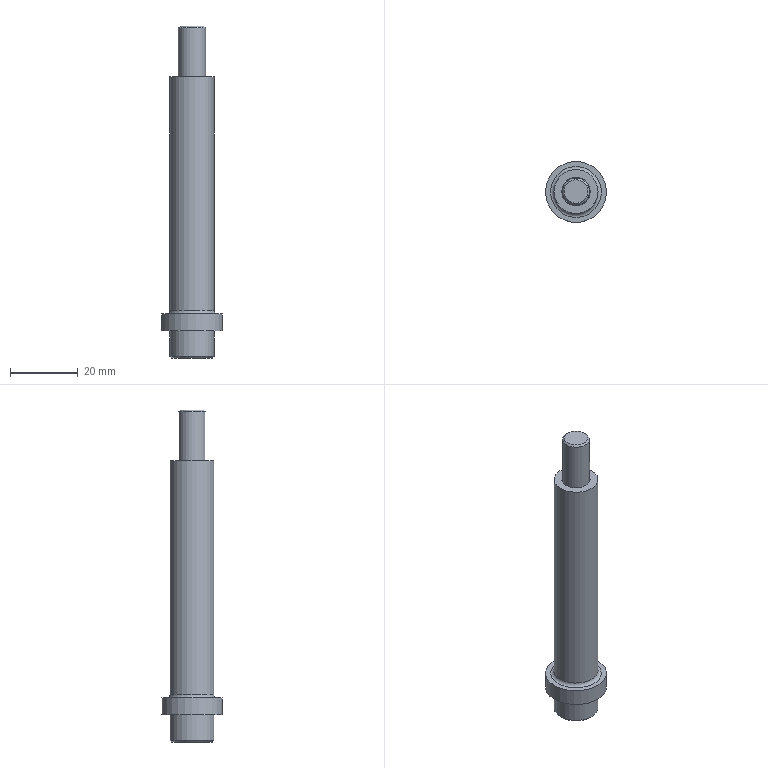Part | NX | features CSR13-60_1 2 | 1 solid | 27 faces | box 18 x 18 x 98 mm | volume 11857 mm3 | plane 18 | cylinder 5 | cone 3 | torus 1 | commonest cylinder face diameters 13 x2 8 x1 8.4 x1 18 x1
STEP:
#1=CARTESIAN_POINT('',(572.,67.,-106.5));
#2=VERTEX_POINT('',#1);
#3=CARTESIAN_POINT('',(563.,67.,-106.5));
#4=DIRECTION('',(0.,0.,-1.));
#5=DIRECTION('',(1.,0.,0.));
#6=AXIS2_PLACEMENT_3D('',#3,#4,#5);
#7=CIRCLE('',#6,9.);
#8=EDGE_CURVE('',#2,#2,#7,.T.);
#9=ORIENTED_EDGE('',*,*,#8,.T.);
#10=EDGE_LOOP('',(#9));
#11=FACE_BOUND('',#10,.T.);
#12=CARTESIAN_POINT('',(569.5,67.,-106.5));
#13=VERTEX_POINT('',#12);
#14=CARTESIAN_POINT('',(563.,67.,-106.5));
#15=DIRECTION('',(0.,0.,1.));
#16=DIRECTION('',(1.,0.,0.));
#17=AXIS2_PLACEMENT_3D('',#14,#15,#16);
#18=CIRCLE('',#17,6.5);
#19=EDGE_CURVE('',#13,#13,#18,.T.);
#20=ORIENTED_EDGE('',*,*,#19,.T.);
#21=EDGE_LOOP('',(#20));
#22=FACE_BOUND('',#21,.T.);
#23=CARTESIAN_POINT('',(563.,67.,-106.5));
#24=DIRECTION('',(0.,0.,-1.));
#25=DIRECTION('',(1.,0.,0.));
#26=AXIS2_PLACEMENT_3D('',#23,#24,#25);
#27=PLANE('',#26);
#28=ADVANCED_FACE('',(#11,#22),#27,.T.);
#29=CARTESIAN_POINT('',(569.5,67.,-100.5));
#30=VERTEX_POINT('',#29);
#31=CARTESIAN_POINT('',(563.,67.,-100.5));
#32=DIRECTION('',(0.,0.,-1.));
#33=DIRECTION('',(-1.,0.,0.));
#34=AXIS2_PLACEMENT_3D('',#31,#32,#33);
#35=CIRCLE('',#34,6.5);
#36=EDGE_CURVE('',#30,#30,#35,.T.);
#37=ORIENTED_EDGE('',*,*,#36,.F.);
#38=EDGE_LOOP('',(#37));
#39=FACE_BOUND('',#38,.T.);
#40=CARTESIAN_POINT('',(569.5,67.,-31.5));
#41=VERTEX_POINT('',#40);
#42=CARTESIAN_POINT('',(563.,67.,-31.5));
#43=DIRECTION('',(0.,0.,1.));
#44=DIRECTION('',(1.,0.,0.));
#45=AXIS2_PLACEMENT_3D('',#42,#43,#44);
#46=CIRCLE('',#45,6.5);
#47=EDGE_CURVE('',#41,#41,#46,.T.);
#48=ORIENTED_EDGE('',*,*,#47,.F.);
#49=EDGE_LOOP('',(#48));
#50=FACE_BOUND('',#49,.T.);
#51=CARTESIAN_POINT('',(563.,67.,-61.5));
#52=DIRECTION('',(0.,0.,1.));
#53=DIRECTION('',(-1.,0.,0.));
#54=AXIS2_PLACEMENT_3D('',#51,#52,#53);
#55=CYLINDRICAL_SURFACE('',#54,6.5);
#56=ADVANCED_FACE('',(#39,#50),#55,.T.);
#57=CARTESIAN_POINT('',(567.2,67.,-106.5));
#58=VERTEX_POINT('',#57);
#59=CARTESIAN_POINT('',(563.,67.,-106.5));
#60=DIRECTION('',(0.,0.,1.));
#61=DIRECTION('',(1.,0.,0.));
#62=AXIS2_PLACEMENT_3D('',#59,#60,#61);
#63=CIRCLE('',#62,4.2);
#64=EDGE_CURVE('',#58,#58,#63,.T.);
#65=ORIENTED_EDGE('',*,*,#64,.F.);
#66=EDGE_LOOP('',(#65));
#67=FACE_BOUND('',#66,.T.);
#68=CARTESIAN_POINT('',(567.2,67.,-31.5));
#69=VERTEX_POINT('',#68);
#70=CARTESIAN_POINT('',(563.,67.,-31.5));
#71=DIRECTION('',(0.,0.,-1.));
#72=DIRECTION('',(1.,0.,0.));
#73=AXIS2_PLACEMENT_3D('',#70,#71,#72);
#74=CIRCLE('',#73,4.2);
#75=EDGE_CURVE('',#69,#69,#74,.T.);
#76=ORIENTED_EDGE('',*,*,#75,.F.);
#77=EDGE_LOOP('',(#76));
#78=FACE_BOUND('',#77,.T.);
#79=CARTESIAN_POINT('',(563.,67.,-64.));
#80=DIRECTION('',(0.,0.,1.));
#81=DIRECTION('',(-1.,0.,0.));
#82=AXIS2_PLACEMENT_3D('',#79,#80,#81);
#83=CYLINDRICAL_SURFACE('',#82,4.2);
#84=ADVANCED_FACE('',(#67,#78),#83,.F.);
#85=ORIENTED_EDGE('',*,*,#36,.T.);
#86=EDGE_LOOP('',(#85));
#87=FACE_BOUND('',#86,.T.);
#88=CARTESIAN_POINT('',(570.5,67.,-101.5));
#89=VERTEX_POINT('',#88);
#90=CARTESIAN_POINT('',(563.,67.,-101.5));
#91=DIRECTION('',(0.,0.,1.));
#92=DIRECTION('',(-1.,0.,0.));
#93=AXIS2_PLACEMENT_3D('',#90,#91,#92);
#94=CIRCLE('',#93,7.5);
#95=EDGE_CURVE('',#89,#89,#94,.T.);
#96=ORIENTED_EDGE('',*,*,#95,.T.);
#97=EDGE_LOOP('',(#96));
#98=FACE_BOUND('',#97,.T.);
#99=CARTESIAN_POINT('',(563.,67.,-100.5));
#100=DIRECTION('',(0.,0.,-1.));
#101=DIRECTION('',(1.,0.,0.));
#102=AXIS2_PLACEMENT_3D('',#99,#100,#101);
#103=TOROIDAL_SURFACE('',#102,7.5,1.);
#104=ADVANCED_FACE('',(#87,#98),#103,.F.);
#105=CARTESIAN_POINT('',(572.,67.,-101.5));
#106=VERTEX_POINT('',#105);
#107=CARTESIAN_POINT('',(563.,67.,-101.5));
#108=DIRECTION('',(0.,0.,1.));
#109=DIRECTION('',(1.,0.,0.));
#110=AXIS2_PLACEMENT_3D('',#107,#108,#109);
#111=CIRCLE('',#110,9.);
#112=EDGE_CURVE('',#106,#106,#111,.T.);
#113=ORIENTED_EDGE('',*,*,#112,.T.);
#114=EDGE_LOOP('',(#113));
#115=FACE_BOUND('',#114,.T.);
#116=ORIENTED_EDGE('',*,*,#95,.F.);
#117=EDGE_LOOP('',(#116));
#118=FACE_BOUND('',#117,.T.);
#119=CARTESIAN_POINT('',(563.,67.,-101.5));
#120=DIRECTION('',(0.,0.,1.));
#121=DIRECTION('',(-1.,0.,0.));
#122=AXIS2_PLACEMENT_3D('',#119,#120,#121);
#123=PLANE('',#122);
#124=ADVANCED_FACE('',(#115,#118),#123,.T.);
#125=ORIENTED_EDGE('',*,*,#75,.T.);
#126=EDGE_LOOP('',(#125));
#127=FACE_BOUND('',#126,.T.);
#128=ORIENTED_EDGE('',*,*,#47,.T.);
#129=EDGE_LOOP('',(#128));
#130=FACE_BOUND('',#129,.T.);
#131=CARTESIAN_POINT('',(563.,67.,-31.5));
#132=DIRECTION('',(0.,0.,1.));
#133=DIRECTION('',(-1.,0.,0.));
#134=AXIS2_PLACEMENT_3D('',#131,#132,#133);
#135=PLANE('',#134);
#136=ADVANCED_FACE('',(#127,#130),#135,.T.);
#137=ORIENTED_EDGE('',*,*,#8,.F.);
#138=EDGE_LOOP('',(#137));
#139=FACE_BOUND('',#138,.T.);
#140=ORIENTED_EDGE('',*,*,#112,.F.);
#141=EDGE_LOOP('',(#140));
#142=FACE_BOUND('',#141,.T.);
#143=CARTESIAN_POINT('',(563.,67.,-104.));
#144=DIRECTION('',(0.,0.,1.));
#145=DIRECTION('',(-1.,0.,0.));
#146=AXIS2_PLACEMENT_3D('',#143,#144,#145);
#147=CYLINDRICAL_SURFACE('',#146,9.);
#148=ADVANCED_FACE('',(#139,#142),#147,.T.);
#149=CARTESIAN_POINT('',(563.,63.536,-114.5));
#150=VERTEX_POINT('',#149);
#151=CARTESIAN_POINT('',(566.,65.268,-114.5));
#152=VERTEX_POINT('',#151);
#153=CARTESIAN_POINT('',(564.5,64.402,-114.5));
#154=DIRECTION('',(0.866,0.5,0.));
#155=VECTOR('',#154,1000.);
#156=LINE('',#153,#155);
#157=EDGE_CURVE('',#150,#152,#156,.T.);
#158=ORIENTED_EDGE('',*,*,#157,.T.);
#159=CARTESIAN_POINT('',(566.,68.732,-114.5));
#160=VERTEX_POINT('',#159);
#161=CARTESIAN_POINT('',(566.,67.,-114.5));
#162=DIRECTION('',(0.,1.,0.));
#163=VECTOR('',#162,1000.);
#164=LINE('',#161,#163);
#165=EDGE_CURVE('',#152,#160,#164,.T.);
#166=ORIENTED_EDGE('',*,*,#165,.T.);
#167=CARTESIAN_POINT('',(563.,70.464,-114.5));
#168=VERTEX_POINT('',#167);
#169=CARTESIAN_POINT('',(564.5,69.598,-114.5));
#170=DIRECTION('',(-0.866,0.5,0.));
#171=VECTOR('',#170,1000.);
#172=LINE('',#169,#171);
#173=EDGE_CURVE('',#160,#168,#172,.T.);
#174=ORIENTED_EDGE('',*,*,#173,.T.);
#175=CARTESIAN_POINT('',(560.,68.732,-114.5));
#176=VERTEX_POINT('',#175);
#177=CARTESIAN_POINT('',(561.5,69.598,-114.5));
#178=DIRECTION('',(-0.866,-0.5,0.));
#179=VECTOR('',#178,1000.);
#180=LINE('',#177,#179);
#181=EDGE_CURVE('',#168,#176,#180,.T.);
#182=ORIENTED_EDGE('',*,*,#181,.T.);
#183=CARTESIAN_POINT('',(560.,65.268,-114.5));
#184=VERTEX_POINT('',#183);
#185=CARTESIAN_POINT('',(560.,67.,-114.5));
#186=DIRECTION('',(0.,-1.,0.));
#187=VECTOR('',#186,1000.);
#188=LINE('',#185,#187);
#189=EDGE_CURVE('',#176,#184,#188,.T.);
#190=ORIENTED_EDGE('',*,*,#189,.T.);
#191=CARTESIAN_POINT('',(561.5,64.402,-114.5));
#192=DIRECTION('',(0.866,-0.5,0.));
#193=VECTOR('',#192,1000.);
#194=LINE('',#191,#193);
#195=EDGE_CURVE('',#184,#150,#194,.T.);
#196=ORIENTED_EDGE('',*,*,#195,.T.);
#197=EDGE_LOOP('',(#158,#166,#174,#182,#190,#196));
#198=FACE_BOUND('',#197,.T.);
#199=CARTESIAN_POINT('',(569.,67.,-114.5));
#200=VERTEX_POINT('',#199);
#201=CARTESIAN_POINT('',(563.,67.,-114.5));
#202=DIRECTION('',(0.,0.,1.));
#203=DIRECTION('',(-1.,0.,0.));
#204=AXIS2_PLACEMENT_3D('',#201,#202,#203);
#205=CIRCLE('',#204,6.);
#206=EDGE_CURVE('',#200,#200,#205,.T.);
#207=ORIENTED_EDGE('',*,*,#206,.F.);
#208=EDGE_LOOP('',(#207));
#209=FACE_BOUND('',#208,.T.);
#210=CARTESIAN_POINT('',(563.,67.,-114.5));
#211=DIRECTION('',(0.,0.,-1.));
#212=DIRECTION('',(1.,0.,0.));
#213=AXIS2_PLACEMENT_3D('',#210,#211,#212);
#214=PLANE('',#213);
#215=ADVANCED_FACE('',(#198,#209),#214,.T.);
#216=ORIENTED_EDGE('',*,*,#19,.F.);
#217=EDGE_LOOP('',(#216));
#218=FACE_BOUND('',#217,.T.);
#219=CARTESIAN_POINT('',(569.5,67.,-114.));
#220=VERTEX_POINT('',#219);
#221=CARTESIAN_POINT('',(563.,67.,-114.));
#222=DIRECTION('',(0.,0.,-1.));
#223=DIRECTION('',(-1.,0.,0.));
#224=AXIS2_PLACEMENT_3D('',#221,#222,#223);
#225=CIRCLE('',#224,6.5);
#226=EDGE_CURVE('',#220,#220,#225,.T.);
#227=ORIENTED_EDGE('',*,*,#226,.F.);
#228=EDGE_LOOP('',(#227));
#229=FACE_BOUND('',#228,.T.);
#230=CARTESIAN_POINT('',(563.,67.,-110.5));
#231=DIRECTION('',(0.,0.,1.));
#232=DIRECTION('',(-1.,0.,0.));
#233=AXIS2_PLACEMENT_3D('',#230,#231,#232);
#234=CYLINDRICAL_SURFACE('',#233,6.5);
#235=ADVANCED_FACE('',(#218,#229),#234,.T.);
#236=ORIENTED_EDGE('',*,*,#226,.T.);
#237=EDGE_LOOP('',(#236));
#238=FACE_BOUND('',#237,.T.);
#239=ORIENTED_EDGE('',*,*,#206,.T.);
#240=EDGE_LOOP('',(#239));
#241=FACE_BOUND('',#240,.T.);
#242=CARTESIAN_POINT('',(563.,67.,-114.5));
#243=DIRECTION('',(0.,0.,1.));
#244=DIRECTION('',(1.,0.,0.));
#245=AXIS2_PLACEMENT_3D('',#242,#243,#244);
#246=CONICAL_SURFACE('',#245,6.,0.7854);
#247=ADVANCED_FACE('',(#238,#241),#246,.T.);
#248=CARTESIAN_POINT('',(566.,65.268,-110.5));
#249=VERTEX_POINT('',#248);
#250=CARTESIAN_POINT('',(566.,65.268,-112.5));
#251=DIRECTION('',(0.,0.,-1.));
#252=VECTOR('',#251,1000.);
#253=LINE('',#250,#252);
#254=EDGE_CURVE('',#249,#152,#253,.T.);
#255=ORIENTED_EDGE('',*,*,#254,.F.);
#256=CARTESIAN_POINT('',(566.,68.732,-110.5));
#257=VERTEX_POINT('',#256);
#258=CARTESIAN_POINT('',(566.,67.,-110.5));
#259=DIRECTION('',(0.,1.,0.));
#260=VECTOR('',#259,1000.);
#261=LINE('',#258,#260);
#262=EDGE_CURVE('',#249,#257,#261,.T.);
#263=ORIENTED_EDGE('',*,*,#262,.T.);
#264=CARTESIAN_POINT('',(566.,68.732,-112.5));
#265=DIRECTION('',(0.,0.,-1.));
#266=VECTOR('',#265,1000.);
#267=LINE('',#264,#266);
#268=EDGE_CURVE('',#257,#160,#267,.T.);
#269=ORIENTED_EDGE('',*,*,#268,.T.);
#270=ORIENTED_EDGE('',*,*,#165,.F.);
#271=EDGE_LOOP('',(#255,#263,#269,#270));
#272=FACE_BOUND('',#271,.T.);
#273=CARTESIAN_POINT('',(566.,67.,-112.5));
#274=DIRECTION('',(-1.,0.,0.));
#275=DIRECTION('',(0.,0.,-1.));
#276=AXIS2_PLACEMENT_3D('',#273,#274,#275);
#277=PLANE('',#276);
#278=ADVANCED_FACE('',(#272),#277,.T.);
#279=ORIENTED_EDGE('',*,*,#268,.F.);
#280=CARTESIAN_POINT('',(563.,70.464,-110.5));
#281=VERTEX_POINT('',#280);
#282=CARTESIAN_POINT('',(564.5,69.598,-110.5));
#283=DIRECTION('',(-0.866,0.5,0.));
#284=VECTOR('',#283,1000.);
#285=LINE('',#282,#284);
#286=EDGE_CURVE('',#257,#281,#285,.T.);
#287=ORIENTED_EDGE('',*,*,#286,.T.);
#288=CARTESIAN_POINT('',(563.,70.464,-112.5));
#289=DIRECTION('',(0.,0.,-1.));
#290=VECTOR('',#289,1000.);
#291=LINE('',#288,#290);
#292=EDGE_CURVE('',#281,#168,#291,.T.);
#293=ORIENTED_EDGE('',*,*,#292,.T.);
#294=ORIENTED_EDGE('',*,*,#173,.F.);
#295=EDGE_LOOP('',(#279,#287,#293,#294));
#296=FACE_BOUND('',#295,.T.);
#297=CARTESIAN_POINT('',(564.5,69.598,-112.5));
#298=DIRECTION('',(-0.5,-0.866,0.));
#299=DIRECTION('',(0.,0.,-1.));
#300=AXIS2_PLACEMENT_3D('',#297,#298,#299);
#301=PLANE('',#300);
#302=ADVANCED_FACE('',(#296),#301,.T.);
#303=ORIENTED_EDGE('',*,*,#292,.F.);
#304=CARTESIAN_POINT('',(560.,68.732,-110.5));
#305=VERTEX_POINT('',#304);
#306=CARTESIAN_POINT('',(561.5,69.598,-110.5));
#307=DIRECTION('',(-0.866,-0.5,0.));
#308=VECTOR('',#307,1000.);
#309=LINE('',#306,#308);
#310=EDGE_CURVE('',#281,#305,#309,.T.);
#311=ORIENTED_EDGE('',*,*,#310,.T.);
#312=CARTESIAN_POINT('',(560.,68.732,-112.5));
#313=DIRECTION('',(0.,0.,-1.));
#314=VECTOR('',#313,1000.);
#315=LINE('',#312,#314);
#316=EDGE_CURVE('',#305,#176,#315,.T.);
#317=ORIENTED_EDGE('',*,*,#316,.T.);
#318=ORIENTED_EDGE('',*,*,#181,.F.);
#319=EDGE_LOOP('',(#303,#311,#317,#318));
#320=FACE_BOUND('',#319,.T.);
#321=CARTESIAN_POINT('',(561.5,69.598,-112.5));
#322=DIRECTION('',(0.5,-0.866,0.));
#323=DIRECTION('',(0.,0.,1.));
#324=AXIS2_PLACEMENT_3D('',#321,#322,#323);
#325=PLANE('',#324);
#326=ADVANCED_FACE('',(#320),#325,.T.);
#327=ORIENTED_EDGE('',*,*,#316,.F.);
#328=CARTESIAN_POINT('',(560.,65.268,-110.5));
#329=VERTEX_POINT('',#328);
#330=CARTESIAN_POINT('',(560.,67.,-110.5));
#331=DIRECTION('',(0.,-1.,0.));
#332=VECTOR('',#331,1000.);
#333=LINE('',#330,#332);
#334=EDGE_CURVE('',#305,#329,#333,.T.);
#335=ORIENTED_EDGE('',*,*,#334,.T.);
#336=CARTESIAN_POINT('',(560.,65.268,-112.5));
#337=DIRECTION('',(0.,0.,-1.));
#338=VECTOR('',#337,1000.);
#339=LINE('',#336,#338);
#340=EDGE_CURVE('',#329,#184,#339,.T.);
#341=ORIENTED_EDGE('',*,*,#340,.T.);
#342=ORIENTED_EDGE('',*,*,#189,.F.);
#343=EDGE_LOOP('',(#327,#335,#341,#342));
#344=FACE_BOUND('',#343,.T.);
#345=CARTESIAN_POINT('',(560.,67.,-112.5));
#346=DIRECTION('',(1.,0.,0.));
#347=DIRECTION('',(0.,0.,1.));
#348=AXIS2_PLACEMENT_3D('',#345,#346,#347);
#349=PLANE('',#348);
#350=ADVANCED_FACE('',(#344),#349,.T.);
#351=ORIENTED_EDGE('',*,*,#340,.F.);
#352=CARTESIAN_POINT('',(563.,63.536,-110.5));
#353=VERTEX_POINT('',#352);
#354=CARTESIAN_POINT('',(561.5,64.402,-110.5));
#355=DIRECTION('',(0.866,-0.5,0.));
#356=VECTOR('',#355,1000.);
#357=LINE('',#354,#356);
#358=EDGE_CURVE('',#329,#353,#357,.T.);
#359=ORIENTED_EDGE('',*,*,#358,.T.);
#360=CARTESIAN_POINT('',(563.,63.536,-112.5));
#361=DIRECTION('',(0.,0.,-1.));
#362=VECTOR('',#361,1000.);
#363=LINE('',#360,#362);
#364=EDGE_CURVE('',#353,#150,#363,.T.);
#365=ORIENTED_EDGE('',*,*,#364,.T.);
#366=ORIENTED_EDGE('',*,*,#195,.F.);
#367=EDGE_LOOP('',(#351,#359,#365,#366));
#368=FACE_BOUND('',#367,.T.);
#369=CARTESIAN_POINT('',(561.5,64.402,-112.5));
#370=DIRECTION('',(0.5,0.866,0.));
#371=DIRECTION('',(0.,0.,1.));
#372=AXIS2_PLACEMENT_3D('',#369,#370,#371);
#373=PLANE('',#372);
#374=ADVANCED_FACE('',(#368),#373,.T.);
#375=ORIENTED_EDGE('',*,*,#364,.F.);
#376=CARTESIAN_POINT('',(564.5,64.402,-110.5));
#377=DIRECTION('',(0.866,0.5,0.));
#378=VECTOR('',#377,1000.);
#379=LINE('',#376,#378);
#380=EDGE_CURVE('',#353,#249,#379,.T.);
#381=ORIENTED_EDGE('',*,*,#380,.T.);
#382=ORIENTED_EDGE('',*,*,#254,.T.);
#383=ORIENTED_EDGE('',*,*,#157,.F.);
#384=EDGE_LOOP('',(#375,#381,#382,#383));
#385=FACE_BOUND('',#384,.T.);
#386=CARTESIAN_POINT('',(564.5,64.402,-112.5));
#387=DIRECTION('',(-0.5,0.866,0.));
#388=DIRECTION('',(0.,0.,-1.));
#389=AXIS2_PLACEMENT_3D('',#386,#387,#388);
#390=PLANE('',#389);
#391=ADVANCED_FACE('',(#385),#390,.T.);
#392=CARTESIAN_POINT('',(563.,67.,-110.5));
#393=DIRECTION('',(0.,0.,-1.));
#394=DIRECTION('',(1.,0.,0.));
#395=AXIS2_PLACEMENT_3D('',#392,#393,#394);
#396=CIRCLE('',#395,3.464);
#397=EDGE_CURVE('',#257,#249,#396,.T.);
#398=ORIENTED_EDGE('',*,*,#397,.T.);
#399=CARTESIAN_POINT('',(563.,67.,-110.5));
#400=DIRECTION('',(0.,0.,-1.));
#401=DIRECTION('',(1.,0.,0.));
#402=AXIS2_PLACEMENT_3D('',#399,#400,#401);
#403=CIRCLE('',#402,3.464);
#404=EDGE_CURVE('',#249,#353,#403,.T.);
#405=ORIENTED_EDGE('',*,*,#404,.T.);
#406=CARTESIAN_POINT('',(563.,67.,-110.5));
#407=DIRECTION('',(0.,0.,-1.));
#408=DIRECTION('',(1.,0.,0.));
#409=AXIS2_PLACEMENT_3D('',#406,#407,#408);
#410=CIRCLE('',#409,3.464);
#411=EDGE_CURVE('',#353,#329,#410,.T.);
#412=ORIENTED_EDGE('',*,*,#411,.T.);
#413=CARTESIAN_POINT('',(563.,67.,-110.5));
#414=DIRECTION('',(0.,0.,-1.));
#415=DIRECTION('',(1.,0.,0.));
#416=AXIS2_PLACEMENT_3D('',#413,#414,#415);
#417=CIRCLE('',#416,3.464);
#418=EDGE_CURVE('',#329,#305,#417,.T.);
#419=ORIENTED_EDGE('',*,*,#418,.T.);
#420=CARTESIAN_POINT('',(563.,67.,-110.5));
#421=DIRECTION('',(0.,0.,-1.));
#422=DIRECTION('',(1.,0.,0.));
#423=AXIS2_PLACEMENT_3D('',#420,#421,#422);
#424=CIRCLE('',#423,3.464);
#425=EDGE_CURVE('',#305,#281,#424,.T.);
#426=ORIENTED_EDGE('',*,*,#425,.T.);
#427=CARTESIAN_POINT('',(563.,67.,-110.5));
#428=DIRECTION('',(0.,0.,-1.));
#429=DIRECTION('',(1.,0.,0.));
#430=AXIS2_PLACEMENT_3D('',#427,#428,#429);
#431=CIRCLE('',#430,3.464);
#432=EDGE_CURVE('',#281,#257,#431,.T.);
#433=ORIENTED_EDGE('',*,*,#432,.T.);
#434=EDGE_LOOP('',(#398,#405,#412,#419,#426,#433));
#435=FACE_BOUND('',#434,.T.);
#436=CARTESIAN_POINT('',(563.,67.,-109.5));
#437=VERTEX_POINT('',#436);
#438=VERTEX_LOOP('',#437);
#439=FACE_BOUND('',#438,.T.);
#440=CARTESIAN_POINT('',(563.,67.,-110.));
#441=DIRECTION('',(0.,0.,-1.));
#442=DIRECTION('',(-1.,0.,0.));
#443=AXIS2_PLACEMENT_3D('',#440,#441,#442);
#444=CONICAL_SURFACE('',#443,1.732,1.29);
#445=ADVANCED_FACE('',(#435,#439),#444,.F.);
#446=ORIENTED_EDGE('',*,*,#358,.F.);
#447=ORIENTED_EDGE('',*,*,#411,.F.);
#448=EDGE_LOOP('',(#446,#447));
#449=FACE_BOUND('',#448,.T.);
#450=CARTESIAN_POINT('',(563.,67.,-110.5));
#451=DIRECTION('',(0.,0.,-1.));
#452=DIRECTION('',(1.,0.,0.));
#453=AXIS2_PLACEMENT_3D('',#450,#451,#452);
#454=PLANE('',#453);
#455=ADVANCED_FACE('',(#449),#454,.F.);
#456=ORIENTED_EDGE('',*,*,#334,.F.);
#457=ORIENTED_EDGE('',*,*,#418,.F.);
#458=EDGE_LOOP('',(#456,#457));
#459=FACE_BOUND('',#458,.T.);
#460=CARTESIAN_POINT('',(563.,67.,-110.5));
#461=DIRECTION('',(0.,0.,-1.));
#462=DIRECTION('',(1.,0.,0.));
#463=AXIS2_PLACEMENT_3D('',#460,#461,#462);
#464=PLANE('',#463);
#465=ADVANCED_FACE('',(#459),#464,.F.);
#466=ORIENTED_EDGE('',*,*,#310,.F.);
#467=ORIENTED_EDGE('',*,*,#425,.F.);
#468=EDGE_LOOP('',(#466,#467));
#469=FACE_BOUND('',#468,.T.);
#470=CARTESIAN_POINT('',(563.,67.,-110.5));
#471=DIRECTION('',(0.,0.,-1.));
#472=DIRECTION('',(1.,0.,0.));
#473=AXIS2_PLACEMENT_3D('',#470,#471,#472);
#474=PLANE('',#473);
#475=ADVANCED_FACE('',(#469),#474,.F.);
#476=ORIENTED_EDGE('',*,*,#286,.F.);
#477=ORIENTED_EDGE('',*,*,#432,.F.);
#478=EDGE_LOOP('',(#476,#477));
#479=FACE_BOUND('',#478,.T.);
#480=CARTESIAN_POINT('',(563.,67.,-110.5));
#481=DIRECTION('',(0.,0.,-1.));
#482=DIRECTION('',(1.,0.,0.));
#483=AXIS2_PLACEMENT_3D('',#480,#481,#482);
#484=PLANE('',#483);
#485=ADVANCED_FACE('',(#479),#484,.F.);
#486=ORIENTED_EDGE('',*,*,#262,.F.);
#487=ORIENTED_EDGE('',*,*,#397,.F.);
#488=EDGE_LOOP('',(#486,#487));
#489=FACE_BOUND('',#488,.T.);
#490=CARTESIAN_POINT('',(563.,67.,-110.5));
#491=DIRECTION('',(0.,0.,-1.));
#492=DIRECTION('',(1.,0.,0.));
#493=AXIS2_PLACEMENT_3D('',#490,#491,#492);
#494=PLANE('',#493);
#495=ADVANCED_FACE('',(#489),#494,.F.);
#496=ORIENTED_EDGE('',*,*,#380,.F.);
#497=ORIENTED_EDGE('',*,*,#404,.F.);
#498=EDGE_LOOP('',(#496,#497));
#499=FACE_BOUND('',#498,.T.);
#500=CARTESIAN_POINT('',(563.,67.,-110.5));
#501=DIRECTION('',(0.,0.,-1.));
#502=DIRECTION('',(1.,0.,0.));
#503=AXIS2_PLACEMENT_3D('',#500,#501,#502);
#504=PLANE('',#503);
#505=ADVANCED_FACE('',(#499),#504,.F.);
#506=CARTESIAN_POINT('',(567.,67.,-17.));
#507=VERTEX_POINT('',#506);
#508=CARTESIAN_POINT('',(563.,67.,-17.));
#509=DIRECTION('',(0.,0.,1.));
#510=DIRECTION('',(-1.,0.,0.));
#511=AXIS2_PLACEMENT_3D('',#508,#509,#510);
#512=CIRCLE('',#511,4.);
#513=EDGE_CURVE('',#507,#507,#512,.T.);
#514=ORIENTED_EDGE('',*,*,#513,.T.);
#515=EDGE_LOOP('',(#514));
#516=FACE_BOUND('',#515,.T.);
#517=CARTESIAN_POINT('',(566.5,67.,-16.5));
#518=VERTEX_POINT('',#517);
#519=CARTESIAN_POINT('',(563.,67.,-16.5));
#520=DIRECTION('',(0.,0.,-1.));
#521=DIRECTION('',(-1.,0.,0.));
#522=AXIS2_PLACEMENT_3D('',#519,#520,#521);
#523=CIRCLE('',#522,3.5);
#524=EDGE_CURVE('',#518,#518,#523,.T.);
#525=ORIENTED_EDGE('',*,*,#524,.T.);
#526=EDGE_LOOP('',(#525));
#527=FACE_BOUND('',#526,.T.);
#528=CARTESIAN_POINT('',(563.,67.,-16.5));
#529=DIRECTION('',(0.,0.,-1.));
#530=DIRECTION('',(1.,0.,0.));
#531=AXIS2_PLACEMENT_3D('',#528,#529,#530);
#532=CONICAL_SURFACE('',#531,3.5,0.7854);
#533=ADVANCED_FACE('',(#516,#527),#532,.T.);
#534=CARTESIAN_POINT('',(567.,67.,-106.5));
#535=VERTEX_POINT('',#534);
#536=CARTESIAN_POINT('',(563.,67.,-106.5));
#537=DIRECTION('',(0.,0.,-1.));
#538=DIRECTION('',(1.,0.,0.));
#539=AXIS2_PLACEMENT_3D('',#536,#537,#538);
#540=CIRCLE('',#539,4.);
#541=EDGE_CURVE('',#535,#535,#540,.T.);
#542=ORIENTED_EDGE('',*,*,#541,.F.);
#543=EDGE_LOOP('',(#542));
#544=FACE_BOUND('',#543,.T.);
#545=ORIENTED_EDGE('',*,*,#513,.F.);
#546=EDGE_LOOP('',(#545));
#547=FACE_BOUND('',#546,.T.);
#548=CARTESIAN_POINT('',(563.,67.,-56.5));
#549=DIRECTION('',(0.,0.,1.));
#550=DIRECTION('',(-1.,0.,0.));
#551=AXIS2_PLACEMENT_3D('',#548,#549,#550);
#552=CYLINDRICAL_SURFACE('',#551,4.);
#553=ADVANCED_FACE('',(#544,#547),#552,.T.);
#554=ORIENTED_EDGE('',*,*,#524,.F.);
#555=EDGE_LOOP('',(#554));
#556=FACE_BOUND('',#555,.T.);
#557=CARTESIAN_POINT('',(563.,67.,-16.5));
#558=DIRECTION('',(0.,0.,1.));
#559=DIRECTION('',(-1.,0.,0.));
#560=AXIS2_PLACEMENT_3D('',#557,#558,#559);
#561=PLANE('',#560);
#562=ADVANCED_FACE('',(#556),#561,.T.);
#563=ORIENTED_EDGE('',*,*,#64,.T.);
#564=EDGE_LOOP('',(#563));
#565=FACE_BOUND('',#564,.T.);
#566=ORIENTED_EDGE('',*,*,#541,.T.);
#567=EDGE_LOOP('',(#566));
#568=FACE_BOUND('',#567,.T.);
#569=CARTESIAN_POINT('',(563.,67.,-106.5));
#570=DIRECTION('',(0.,0.,1.));
#571=DIRECTION('',(-1.,0.,0.));
#572=AXIS2_PLACEMENT_3D('',#569,#570,#571);
#573=PLANE('',#572);
#574=ADVANCED_FACE('',(#565,#568),#573,.T.);
#575=CLOSED_SHELL('',(#28,#56,#84,#104,#124,#136,#148,#215,#235,#247,#278,#302,#326,#350,#374,#391,#445,#455,#465,#475,#485,#495,#505,#533,#553,#562,#574));
#576=MANIFOLD_SOLID_BREP('',#575);
#577=(LENGTH_UNIT()NAMED_UNIT(*)SI_UNIT(.MILLI.,.METRE.));
#578=UNCERTAINTY_MEASURE_WITH_UNIT(LENGTH_MEASURE(0.00001),#577,'','');
#579=(NAMED_UNIT(*)PLANE_ANGLE_UNIT()SI_UNIT($,.RADIAN.));
#580=(NAMED_UNIT(*)SI_UNIT($,.STERADIAN.)SOLID_ANGLE_UNIT());
#581=(GEOMETRIC_REPRESENTATION_CONTEXT(3)GLOBAL_UNCERTAINTY_ASSIGNED_CONTEXT((#578))GLOBAL_UNIT_ASSIGNED_CONTEXT((#577,#579,#580))REPRESENTATION_CONTEXT('',''));
#582=ADVANCED_BREP_SHAPE_REPRESENTATION('',(#576),#581);